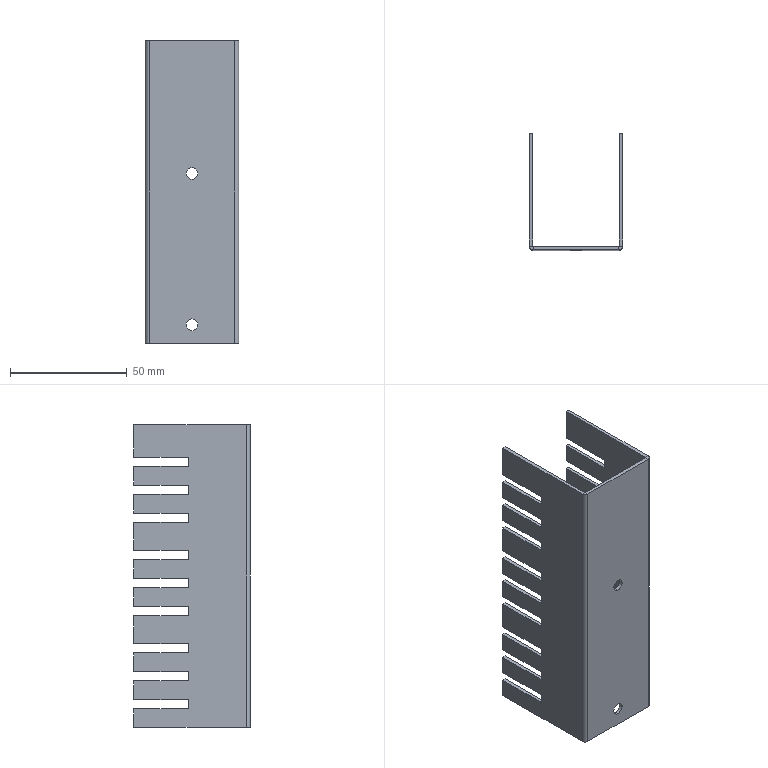Part | SolidWorks | features Cut 1, FlatPattern 1, ICE 1, LPattern 1, SMBaseFlange 1, SheetMetal 1 | 1 solid | 98 faces | box 40 x 50 x 130 mm | volume 23970 mm3 | plane 90 | cylinder 8 | commonest cylinder face diameters 5 x4 0.4 x2 3.4 x2